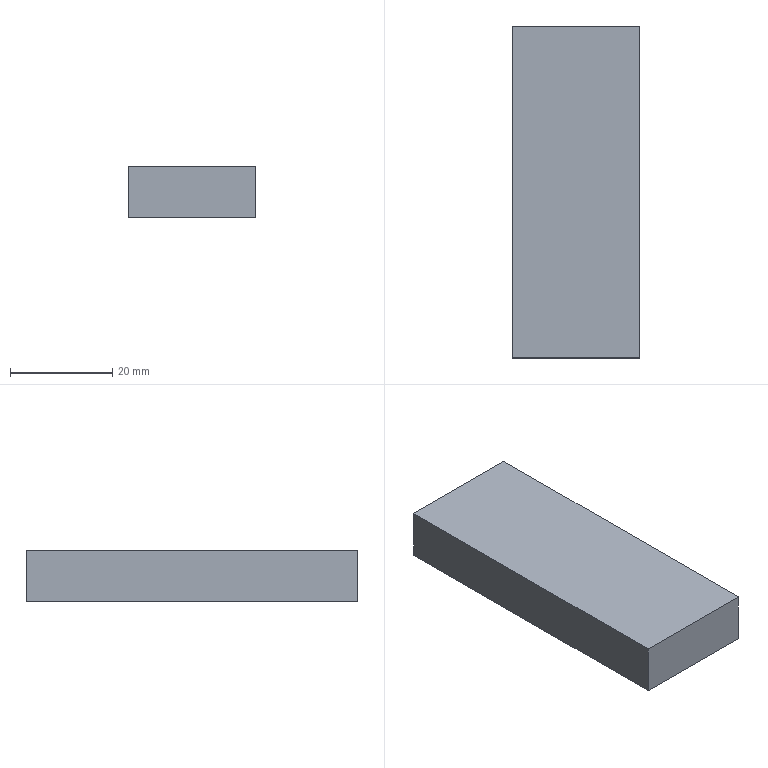Part | NX | features solid 2 | 1 solid | 6 faces | box 25 x 65 x 10 mm | volume 16250 mm3 | plane 6
STEP:
#1=CARTESIAN_POINT('',(520.,375.,20.));
#2=VERTEX_POINT('',#1);
#3=CARTESIAN_POINT('',(545.,375.,20.));
#4=VERTEX_POINT('',#3);
#5=CARTESIAN_POINT('',(540.,375.,20.));
#6=DIRECTION('',(-1.,0.,0.));
#7=VECTOR('',#6,1000.);
#8=LINE('',#5,#7);
#9=EDGE_CURVE('',#2,#4,#8,.F.);
#10=ORIENTED_EDGE('',*,*,#9,.F.);
#11=CARTESIAN_POINT('',(520.,310.,20.));
#12=VERTEX_POINT('',#11);
#13=CARTESIAN_POINT('',(520.,300.,20.));
#14=DIRECTION('',(0.,1.,0.));
#15=VECTOR('',#14,1000.);
#16=LINE('',#13,#15);
#17=EDGE_CURVE('',#12,#2,#16,.T.);
#18=ORIENTED_EDGE('',*,*,#17,.F.);
#19=CARTESIAN_POINT('',(545.,310.,20.));
#20=VERTEX_POINT('',#19);
#21=CARTESIAN_POINT('',(540.,310.,20.));
#22=DIRECTION('',(1.,0.,0.));
#23=VECTOR('',#22,1000.);
#24=LINE('',#21,#23);
#25=EDGE_CURVE('',#12,#20,#24,.T.);
#26=ORIENTED_EDGE('',*,*,#25,.T.);
#27=CARTESIAN_POINT('',(545.,300.,20.));
#28=DIRECTION('',(0.,1.,0.));
#29=VECTOR('',#28,1000.);
#30=LINE('',#27,#29);
#31=EDGE_CURVE('',#20,#4,#30,.T.);
#32=ORIENTED_EDGE('',*,*,#31,.T.);
#33=EDGE_LOOP('',(#10,#18,#26,#32));
#34=FACE_BOUND('',#33,.T.);
#35=CARTESIAN_POINT('',(540.,300.,20.));
#36=DIRECTION('',(0.,0.,-1.));
#37=DIRECTION('',(0.,1.,0.));
#38=AXIS2_PLACEMENT_3D('',#35,#36,#37);
#39=PLANE('',#38);
#40=ADVANCED_FACE('',(#34),#39,.F.);
#41=CARTESIAN_POINT('',(520.,310.,10.));
#42=VERTEX_POINT('',#41);
#43=CARTESIAN_POINT('',(520.,310.,-30.));
#44=DIRECTION('',(0.,0.,1.));
#45=VECTOR('',#44,1000.);
#46=LINE('',#43,#45);
#47=EDGE_CURVE('',#42,#12,#46,.T.);
#48=ORIENTED_EDGE('',*,*,#47,.T.);
#49=ORIENTED_EDGE('',*,*,#17,.T.);
#50=CARTESIAN_POINT('',(520.,375.,10.));
#51=VERTEX_POINT('',#50);
#52=CARTESIAN_POINT('',(520.,375.,-30.));
#53=DIRECTION('',(0.,0.,-1.));
#54=VECTOR('',#53,1000.);
#55=LINE('',#52,#54);
#56=EDGE_CURVE('',#51,#2,#55,.F.);
#57=ORIENTED_EDGE('',*,*,#56,.F.);
#58=CARTESIAN_POINT('',(520.,300.,10.));
#59=DIRECTION('',(0.,-1.,0.));
#60=VECTOR('',#59,1000.);
#61=LINE('',#58,#60);
#62=EDGE_CURVE('',#42,#51,#61,.F.);
#63=ORIENTED_EDGE('',*,*,#62,.F.);
#64=EDGE_LOOP('',(#48,#49,#57,#63));
#65=FACE_BOUND('',#64,.T.);
#66=CARTESIAN_POINT('',(520.,300.,-30.));
#67=DIRECTION('',(-1.,0.,0.));
#68=DIRECTION('',(0.,0.,-1.));
#69=AXIS2_PLACEMENT_3D('',#66,#67,#68);
#70=PLANE('',#69);
#71=ADVANCED_FACE('',(#65),#70,.T.);
#72=CARTESIAN_POINT('',(545.,310.,10.));
#73=VERTEX_POINT('',#72);
#74=CARTESIAN_POINT('',(545.,310.,-30.));
#75=DIRECTION('',(0.,0.,1.));
#76=VECTOR('',#75,1000.);
#77=LINE('',#74,#76);
#78=EDGE_CURVE('',#73,#20,#77,.T.);
#79=ORIENTED_EDGE('',*,*,#78,.F.);
#80=CARTESIAN_POINT('',(545.,375.,10.));
#81=VERTEX_POINT('',#80);
#82=CARTESIAN_POINT('',(545.,300.,10.));
#83=DIRECTION('',(0.,1.,0.));
#84=VECTOR('',#83,1000.);
#85=LINE('',#82,#84);
#86=EDGE_CURVE('',#73,#81,#85,.T.);
#87=ORIENTED_EDGE('',*,*,#86,.T.);
#88=CARTESIAN_POINT('',(545.,375.,-30.));
#89=DIRECTION('',(0.,0.,-1.));
#90=VECTOR('',#89,1000.);
#91=LINE('',#88,#90);
#92=EDGE_CURVE('',#81,#4,#91,.F.);
#93=ORIENTED_EDGE('',*,*,#92,.T.);
#94=ORIENTED_EDGE('',*,*,#31,.F.);
#95=EDGE_LOOP('',(#79,#87,#93,#94));
#96=FACE_BOUND('',#95,.T.);
#97=CARTESIAN_POINT('',(545.,300.,-30.));
#98=DIRECTION('',(-1.,0.,0.));
#99=DIRECTION('',(0.,0.,-1.));
#100=AXIS2_PLACEMENT_3D('',#97,#98,#99);
#101=PLANE('',#100);
#102=ADVANCED_FACE('',(#96),#101,.F.);
#103=ORIENTED_EDGE('',*,*,#47,.F.);
#104=CARTESIAN_POINT('',(540.,310.,10.));
#105=DIRECTION('',(1.,0.,0.));
#106=VECTOR('',#105,1000.);
#107=LINE('',#104,#106);
#108=EDGE_CURVE('',#42,#73,#107,.T.);
#109=ORIENTED_EDGE('',*,*,#108,.T.);
#110=ORIENTED_EDGE('',*,*,#78,.T.);
#111=ORIENTED_EDGE('',*,*,#25,.F.);
#112=EDGE_LOOP('',(#103,#109,#110,#111));
#113=FACE_BOUND('',#112,.T.);
#114=CARTESIAN_POINT('',(540.,310.,-30.));
#115=DIRECTION('',(0.,1.,0.));
#116=DIRECTION('',(0.,0.,1.));
#117=AXIS2_PLACEMENT_3D('',#114,#115,#116);
#118=PLANE('',#117);
#119=ADVANCED_FACE('',(#113),#118,.F.);
#120=ORIENTED_EDGE('',*,*,#92,.F.);
#121=CARTESIAN_POINT('',(540.,375.,10.));
#122=DIRECTION('',(1.,0.,0.));
#123=VECTOR('',#122,1000.);
#124=LINE('',#121,#123);
#125=EDGE_CURVE('',#81,#51,#124,.F.);
#126=ORIENTED_EDGE('',*,*,#125,.T.);
#127=ORIENTED_EDGE('',*,*,#56,.T.);
#128=ORIENTED_EDGE('',*,*,#9,.T.);
#129=EDGE_LOOP('',(#120,#126,#127,#128));
#130=FACE_BOUND('',#129,.T.);
#131=CARTESIAN_POINT('',(540.,375.,-30.));
#132=DIRECTION('',(0.,1.,0.));
#133=DIRECTION('',(0.,0.,1.));
#134=AXIS2_PLACEMENT_3D('',#131,#132,#133);
#135=PLANE('',#134);
#136=ADVANCED_FACE('',(#130),#135,.T.);
#137=ORIENTED_EDGE('',*,*,#62,.T.);
#138=ORIENTED_EDGE('',*,*,#125,.F.);
#139=ORIENTED_EDGE('',*,*,#86,.F.);
#140=ORIENTED_EDGE('',*,*,#108,.F.);
#141=EDGE_LOOP('',(#137,#138,#139,#140));
#142=FACE_BOUND('',#141,.T.);
#143=CARTESIAN_POINT('',(-202.,435.,10.));
#144=DIRECTION('',(0.,0.,1.));
#145=DIRECTION('',(1.,0.,0.));
#146=AXIS2_PLACEMENT_3D('',#143,#144,#145);
#147=PLANE('',#146);
#148=ADVANCED_FACE('',(#142),#147,.F.);
#149=CLOSED_SHELL('',(#40,#71,#102,#119,#136,#148));
#150=MANIFOLD_SOLID_BREP('',#149);
#151=(LENGTH_UNIT()NAMED_UNIT(*)SI_UNIT(.MILLI.,.METRE.));
#152=UNCERTAINTY_MEASURE_WITH_UNIT(LENGTH_MEASURE(0.00001),#151,'','');
#153=(NAMED_UNIT(*)PLANE_ANGLE_UNIT()SI_UNIT($,.RADIAN.));
#154=(NAMED_UNIT(*)SI_UNIT($,.STERADIAN.)SOLID_ANGLE_UNIT());
#155=(GEOMETRIC_REPRESENTATION_CONTEXT(3)GLOBAL_UNCERTAINTY_ASSIGNED_CONTEXT((#152))GLOBAL_UNIT_ASSIGNED_CONTEXT((#151,#153,#154))REPRESENTATION_CONTEXT('',''));
#156=ADVANCED_BREP_SHAPE_REPRESENTATION('',(#150),#155);